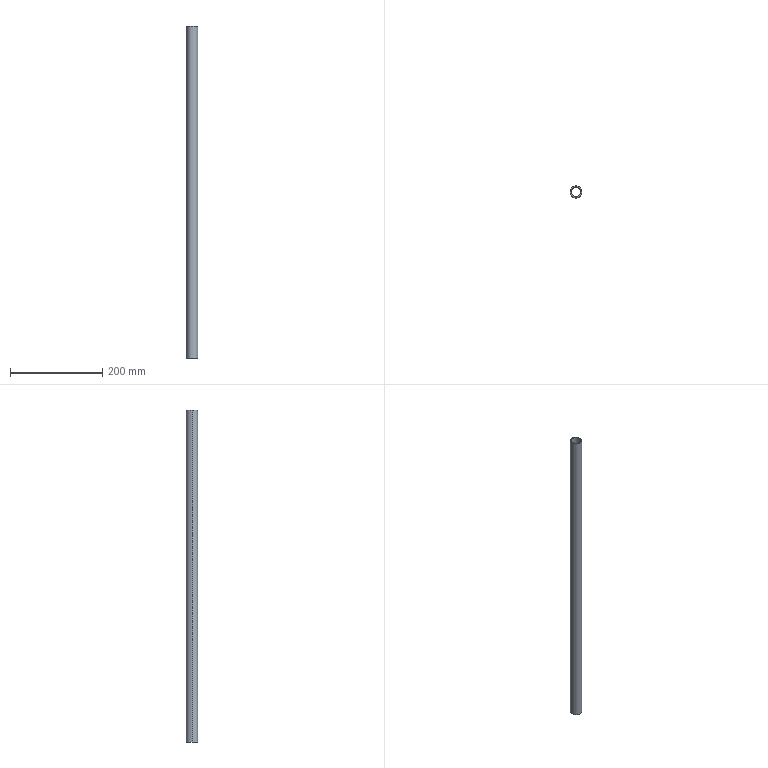Part | SolidWorks | features Extrusion 1 | 1 solid | 6 faces | box 25 x 25 x 720 mm | volume 104050 mm3 | cylinder 4 | plane 2 | commonest cylinder face diameters 21 x2 25 x2
STEP:
#1=CARTESIAN_POINT('',(-10.5,0.,360.));
#2=VERTEX_POINT('',#1);
#3=CARTESIAN_POINT('',(10.5,0.,360.));
#4=VERTEX_POINT('',#3);
#5=CARTESIAN_POINT('',(0.,0.,360.));
#6=DIRECTION('',(0.,0.,1.));
#7=DIRECTION('',(1.,0.,0.));
#8=AXIS2_PLACEMENT_3D('',#5,#6,#7);
#9=CIRCLE('',#8,10.5);
#10=EDGE_CURVE('',#2,#4,#9,.T.);
#11=ORIENTED_EDGE('',*,*,#10,.T.);
#12=CARTESIAN_POINT('',(10.5,0.,-360.));
#13=VERTEX_POINT('',#12);
#14=CARTESIAN_POINT('',(10.5,0.,360.));
#15=DIRECTION('',(0.,0.,-1.));
#16=VECTOR('',#15,1000.);
#17=LINE('',#14,#16);
#18=EDGE_CURVE('',#4,#13,#17,.T.);
#19=ORIENTED_EDGE('',*,*,#18,.T.);
#20=CARTESIAN_POINT('',(-10.5,0.,-360.));
#21=VERTEX_POINT('',#20);
#22=CARTESIAN_POINT('',(0.,0.,-360.));
#23=DIRECTION('',(0.,0.,1.));
#24=DIRECTION('',(1.,0.,0.));
#25=AXIS2_PLACEMENT_3D('',#22,#23,#24);
#26=CIRCLE('',#25,10.5);
#27=EDGE_CURVE('',#21,#13,#26,.T.);
#28=ORIENTED_EDGE('',*,*,#27,.F.);
#29=CARTESIAN_POINT('',(-10.5,0.,360.));
#30=DIRECTION('',(0.,0.,-1.));
#31=VECTOR('',#30,1000.);
#32=LINE('',#29,#31);
#33=EDGE_CURVE('',#2,#21,#32,.T.);
#34=ORIENTED_EDGE('',*,*,#33,.F.);
#35=EDGE_LOOP('',(#11,#19,#28,#34));
#36=FACE_OUTER_BOUND('',#35,.T.);
#37=CARTESIAN_POINT('',(0.,0.,360.));
#38=DIRECTION('',(0.,0.,-1.));
#39=DIRECTION('',(-1.,0.,0.));
#40=AXIS2_PLACEMENT_3D('',#37,#38,#39);
#41=CYLINDRICAL_SURFACE('',#40,10.5);
#42=ADVANCED_FACE('',(#36),#41,.F.);
#43=CARTESIAN_POINT('',(12.5,0.,360.));
#44=VERTEX_POINT('',#43);
#45=CARTESIAN_POINT('',(-12.5,0.,360.));
#46=VERTEX_POINT('',#45);
#47=CARTESIAN_POINT('',(0.,0.,360.));
#48=DIRECTION('',(0.,0.,1.));
#49=DIRECTION('',(1.,0.,0.));
#50=AXIS2_PLACEMENT_3D('',#47,#48,#49);
#51=CIRCLE('',#50,12.5);
#52=EDGE_CURVE('',#44,#46,#51,.T.);
#53=ORIENTED_EDGE('',*,*,#52,.F.);
#54=CARTESIAN_POINT('',(12.5,0.,-360.));
#55=VERTEX_POINT('',#54);
#56=CARTESIAN_POINT('',(12.5,0.,360.));
#57=DIRECTION('',(0.,0.,-1.));
#58=VECTOR('',#57,1000.);
#59=LINE('',#56,#58);
#60=EDGE_CURVE('',#44,#55,#59,.T.);
#61=ORIENTED_EDGE('',*,*,#60,.T.);
#62=CARTESIAN_POINT('',(-12.5,0.,-360.));
#63=VERTEX_POINT('',#62);
#64=CARTESIAN_POINT('',(0.,0.,-360.));
#65=DIRECTION('',(0.,0.,1.));
#66=DIRECTION('',(1.,0.,0.));
#67=AXIS2_PLACEMENT_3D('',#64,#65,#66);
#68=CIRCLE('',#67,12.5);
#69=EDGE_CURVE('',#55,#63,#68,.T.);
#70=ORIENTED_EDGE('',*,*,#69,.T.);
#71=CARTESIAN_POINT('',(-12.5,0.,360.));
#72=DIRECTION('',(0.,0.,-1.));
#73=VECTOR('',#72,1000.);
#74=LINE('',#71,#73);
#75=EDGE_CURVE('',#46,#63,#74,.T.);
#76=ORIENTED_EDGE('',*,*,#75,.F.);
#77=EDGE_LOOP('',(#53,#61,#70,#76));
#78=FACE_OUTER_BOUND('',#77,.T.);
#79=CARTESIAN_POINT('',(0.,0.,360.));
#80=DIRECTION('',(0.,0.,-1.));
#81=DIRECTION('',(-1.,0.,0.));
#82=AXIS2_PLACEMENT_3D('',#79,#80,#81);
#83=CYLINDRICAL_SURFACE('',#82,12.5);
#84=ADVANCED_FACE('',(#78),#83,.T.);
#85=CARTESIAN_POINT('',(0.,0.,360.));
#86=DIRECTION('',(0.,0.,1.));
#87=DIRECTION('',(1.,0.,0.));
#88=AXIS2_PLACEMENT_3D('',#85,#86,#87);
#89=CIRCLE('',#88,12.5);
#90=EDGE_CURVE('',#46,#44,#89,.T.);
#91=ORIENTED_EDGE('',*,*,#90,.T.);
#92=ORIENTED_EDGE('',*,*,#52,.T.);
#93=EDGE_LOOP('',(#91,#92));
#94=FACE_OUTER_BOUND('',#93,.T.);
#95=ORIENTED_EDGE('',*,*,#10,.F.);
#96=CARTESIAN_POINT('',(0.,0.,360.));
#97=DIRECTION('',(0.,0.,1.));
#98=DIRECTION('',(1.,0.,0.));
#99=AXIS2_PLACEMENT_3D('',#96,#97,#98);
#100=CIRCLE('',#99,10.5);
#101=EDGE_CURVE('',#4,#2,#100,.T.);
#102=ORIENTED_EDGE('',*,*,#101,.F.);
#103=EDGE_LOOP('',(#95,#102));
#104=FACE_BOUND('',#103,.T.);
#105=CARTESIAN_POINT('',(0.,0.,360.));
#106=DIRECTION('',(0.,0.,1.));
#107=DIRECTION('',(1.,0.,0.));
#108=AXIS2_PLACEMENT_3D('',#105,#106,#107);
#109=PLANE('',#108);
#110=ADVANCED_FACE('',(#94,#104),#109,.T.);
#111=CARTESIAN_POINT('',(0.,0.,-360.));
#112=DIRECTION('',(0.,0.,1.));
#113=DIRECTION('',(1.,0.,0.));
#114=AXIS2_PLACEMENT_3D('',#111,#112,#113);
#115=CIRCLE('',#114,12.5);
#116=EDGE_CURVE('',#63,#55,#115,.T.);
#117=ORIENTED_EDGE('',*,*,#116,.F.);
#118=ORIENTED_EDGE('',*,*,#69,.F.);
#119=EDGE_LOOP('',(#117,#118));
#120=FACE_OUTER_BOUND('',#119,.T.);
#121=ORIENTED_EDGE('',*,*,#27,.T.);
#122=CARTESIAN_POINT('',(0.,0.,-360.));
#123=DIRECTION('',(0.,0.,1.));
#124=DIRECTION('',(1.,0.,0.));
#125=AXIS2_PLACEMENT_3D('',#122,#123,#124);
#126=CIRCLE('',#125,10.5);
#127=EDGE_CURVE('',#13,#21,#126,.T.);
#128=ORIENTED_EDGE('',*,*,#127,.T.);
#129=EDGE_LOOP('',(#121,#128));
#130=FACE_BOUND('',#129,.T.);
#131=CARTESIAN_POINT('',(0.,0.,-360.));
#132=DIRECTION('',(0.,0.,1.));
#133=DIRECTION('',(1.,0.,0.));
#134=AXIS2_PLACEMENT_3D('',#131,#132,#133);
#135=PLANE('',#134);
#136=ADVANCED_FACE('',(#120,#130),#135,.F.);
#137=ORIENTED_EDGE('',*,*,#60,.F.);
#138=ORIENTED_EDGE('',*,*,#90,.F.);
#139=ORIENTED_EDGE('',*,*,#75,.T.);
#140=ORIENTED_EDGE('',*,*,#116,.T.);
#141=EDGE_LOOP('',(#137,#138,#139,#140));
#142=FACE_OUTER_BOUND('',#141,.T.);
#143=CARTESIAN_POINT('',(0.,0.,360.));
#144=DIRECTION('',(0.,0.,-1.));
#145=DIRECTION('',(-1.,0.,0.));
#146=AXIS2_PLACEMENT_3D('',#143,#144,#145);
#147=CYLINDRICAL_SURFACE('',#146,12.5);
#148=ADVANCED_FACE('',(#142),#147,.T.);
#149=ORIENTED_EDGE('',*,*,#18,.F.);
#150=ORIENTED_EDGE('',*,*,#101,.T.);
#151=ORIENTED_EDGE('',*,*,#33,.T.);
#152=ORIENTED_EDGE('',*,*,#127,.F.);
#153=EDGE_LOOP('',(#149,#150,#151,#152));
#154=FACE_OUTER_BOUND('',#153,.T.);
#155=CARTESIAN_POINT('',(0.,0.,360.));
#156=DIRECTION('',(0.,0.,-1.));
#157=DIRECTION('',(-1.,0.,0.));
#158=AXIS2_PLACEMENT_3D('',#155,#156,#157);
#159=CYLINDRICAL_SURFACE('',#158,10.5);
#160=ADVANCED_FACE('',(#154),#159,.F.);
#161=CLOSED_SHELL('',(#42,#84,#110,#136,#148,#160));
#162=MANIFOLD_SOLID_BREP('',#161);
#163=CARTESIAN_POINT('',(0.,0.,0.));
#164=DIRECTION('',(0.,0.,1.));
#165=DIRECTION('',(1.,0.,0.));
#166=AXIS2_PLACEMENT_3D('',#163,#164,#165);
#167=(LENGTH_UNIT()NAMED_UNIT(*)SI_UNIT(.MILLI.,.METRE.));
#168=UNCERTAINTY_MEASURE_WITH_UNIT(LENGTH_MEASURE(0.00001),#167,'','');
#169=(NAMED_UNIT(*)PLANE_ANGLE_UNIT()SI_UNIT($,.RADIAN.));
#170=(NAMED_UNIT(*)SI_UNIT($,.STERADIAN.)SOLID_ANGLE_UNIT());
#171=(GEOMETRIC_REPRESENTATION_CONTEXT(3)GLOBAL_UNCERTAINTY_ASSIGNED_CONTEXT((#168))GLOBAL_UNIT_ASSIGNED_CONTEXT((#167,#169,#170))REPRESENTATION_CONTEXT('',''));
#172=ADVANCED_BREP_SHAPE_REPRESENTATION('',(#162,#166),#171);